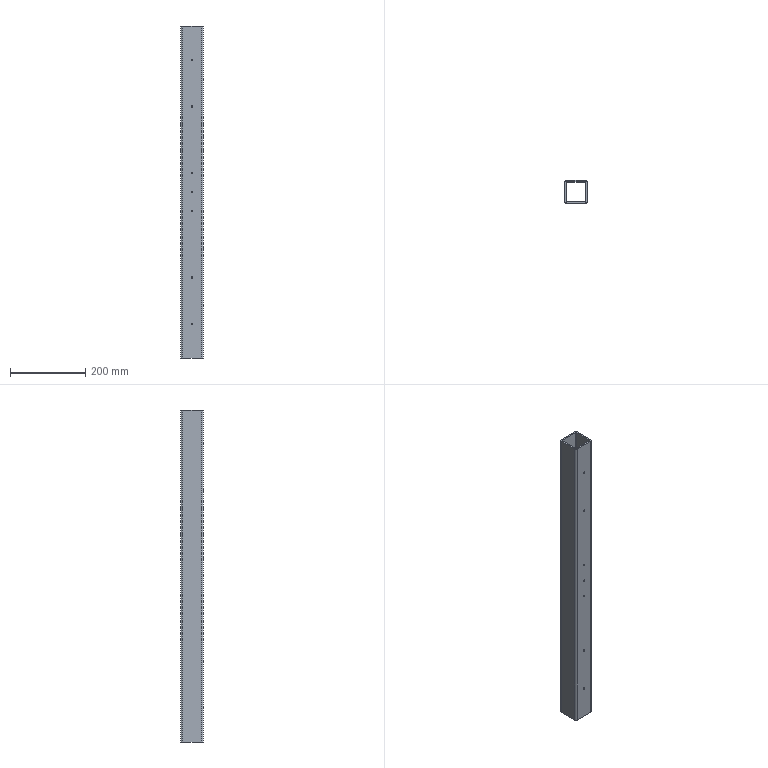Part | STEP file | rear square steel tube 60x60x4x880 | 1 solid | 40 faces | box 60 x 60 x 880 mm | volume 769733 mm3 | cylinder 30 | plane 10 | commonest cylinder face diameters 3.3 x8 5 x8 4.2 x6 2 x4 10 x4